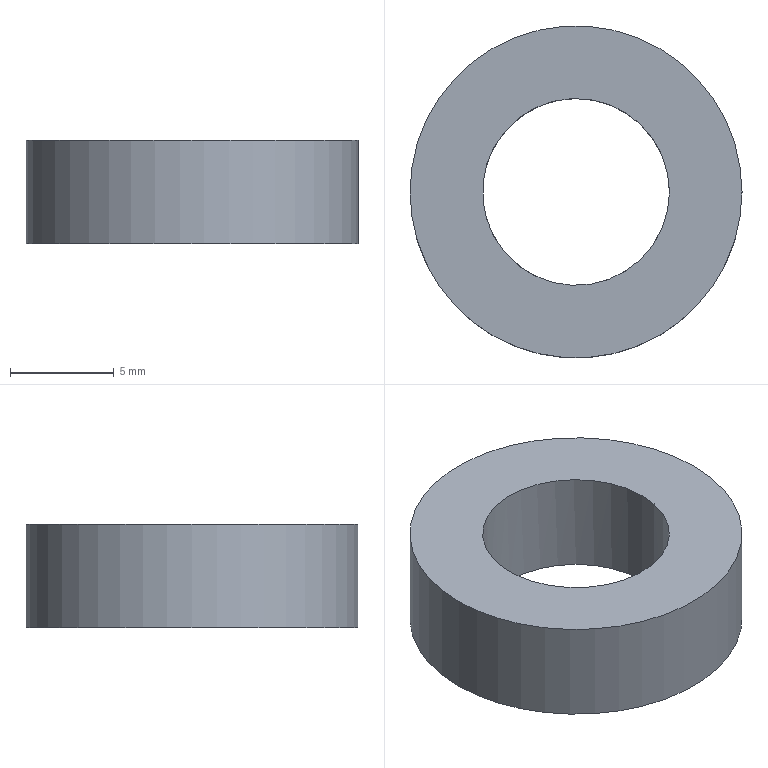Part | NX | features DIE-8 2 | 1 solid | 4 faces | box 16 x 16 x 5 mm | volume 686.728 mm3 | plane 2 | cylinder 2 | commonest cylinder face diameters 9.007 x1 16 x1
STEP:
#1=CARTESIAN_POINT('',(3222.597,-843.322,843.716));
#2=VERTEX_POINT('',#1);
#3=CARTESIAN_POINT('',(3218.094,-843.322,843.716));
#4=DIRECTION('',(0.,0.,1.));
#5=DIRECTION('',(1.,0.,0.));
#6=AXIS2_PLACEMENT_3D('',#3,#4,#5);
#7=CIRCLE('',#6,4.503);
#8=EDGE_CURVE('',#2,#2,#7,.F.);
#9=ORIENTED_EDGE('',*,*,#8,.T.);
#10=EDGE_LOOP('',(#9));
#11=FACE_BOUND('',#10,.T.);
#12=CARTESIAN_POINT('',(3226.094,-843.322,843.716));
#13=VERTEX_POINT('',#12);
#14=CARTESIAN_POINT('',(3218.094,-843.322,843.716));
#15=DIRECTION('',(0.,0.,-1.));
#16=DIRECTION('',(1.,0.,0.));
#17=AXIS2_PLACEMENT_3D('',#14,#15,#16);
#18=CIRCLE('',#17,8.);
#19=EDGE_CURVE('',#13,#13,#18,.T.);
#20=ORIENTED_EDGE('',*,*,#19,.F.);
#21=EDGE_LOOP('',(#20));
#22=FACE_BOUND('',#21,.T.);
#23=CARTESIAN_POINT('',(3218.094,-843.322,843.716));
#24=DIRECTION('',(0.,0.,1.));
#25=DIRECTION('',(1.,0.,0.));
#26=AXIS2_PLACEMENT_3D('',#23,#24,#25);
#27=PLANE('',#26);
#28=ADVANCED_FACE('',(#11,#22),#27,.T.);
#29=CARTESIAN_POINT('',(3213.59,-843.322,838.716));
#30=VERTEX_POINT('',#29);
#31=CARTESIAN_POINT('',(3218.094,-843.322,838.716));
#32=DIRECTION('',(0.,0.,-1.));
#33=DIRECTION('',(-1.,0.,0.));
#34=AXIS2_PLACEMENT_3D('',#31,#32,#33);
#35=CIRCLE('',#34,4.503);
#36=EDGE_CURVE('',#30,#30,#35,.T.);
#37=ORIENTED_EDGE('',*,*,#36,.F.);
#38=EDGE_LOOP('',(#37));
#39=FACE_BOUND('',#38,.T.);
#40=CARTESIAN_POINT('',(3226.094,-843.322,838.716));
#41=VERTEX_POINT('',#40);
#42=CARTESIAN_POINT('',(3218.094,-843.322,838.716));
#43=DIRECTION('',(0.,0.,1.));
#44=DIRECTION('',(1.,0.,0.));
#45=AXIS2_PLACEMENT_3D('',#42,#43,#44);
#46=CIRCLE('',#45,8.);
#47=EDGE_CURVE('',#41,#41,#46,.T.);
#48=ORIENTED_EDGE('',*,*,#47,.F.);
#49=EDGE_LOOP('',(#48));
#50=FACE_BOUND('',#49,.T.);
#51=CARTESIAN_POINT('',(3218.094,-843.322,838.716));
#52=DIRECTION('',(0.,0.,-1.));
#53=DIRECTION('',(-1.,0.,0.));
#54=AXIS2_PLACEMENT_3D('',#51,#52,#53);
#55=PLANE('',#54);
#56=ADVANCED_FACE('',(#39,#50),#55,.T.);
#57=ORIENTED_EDGE('',*,*,#19,.T.);
#58=EDGE_LOOP('',(#57));
#59=FACE_BOUND('',#58,.T.);
#60=ORIENTED_EDGE('',*,*,#47,.T.);
#61=EDGE_LOOP('',(#60));
#62=FACE_BOUND('',#61,.T.);
#63=CARTESIAN_POINT('',(3218.094,-843.322,838.716));
#64=DIRECTION('',(0.,0.,1.));
#65=DIRECTION('',(1.,0.,0.));
#66=AXIS2_PLACEMENT_3D('',#63,#64,#65);
#67=CYLINDRICAL_SURFACE('',#66,8.);
#68=ADVANCED_FACE('',(#59,#62),#67,.T.);
#69=ORIENTED_EDGE('',*,*,#36,.T.);
#70=EDGE_LOOP('',(#69));
#71=FACE_BOUND('',#70,.T.);
#72=ORIENTED_EDGE('',*,*,#8,.F.);
#73=EDGE_LOOP('',(#72));
#74=FACE_BOUND('',#73,.T.);
#75=CARTESIAN_POINT('',(3218.094,-843.322,843.716));
#76=DIRECTION('',(0.,0.,-1.));
#77=DIRECTION('',(1.,0.,0.));
#78=AXIS2_PLACEMENT_3D('',#75,#76,#77);
#79=CYLINDRICAL_SURFACE('',#78,4.503);
#80=ADVANCED_FACE('',(#71,#74),#79,.F.);
#81=CLOSED_SHELL('',(#28,#56,#68,#80));
#82=MANIFOLD_SOLID_BREP('',#81);
#83=(LENGTH_UNIT()NAMED_UNIT(*)SI_UNIT(.MILLI.,.METRE.));
#84=UNCERTAINTY_MEASURE_WITH_UNIT(LENGTH_MEASURE(0.00001),#83,'','');
#85=(NAMED_UNIT(*)PLANE_ANGLE_UNIT()SI_UNIT($,.RADIAN.));
#86=(NAMED_UNIT(*)SI_UNIT($,.STERADIAN.)SOLID_ANGLE_UNIT());
#87=(GEOMETRIC_REPRESENTATION_CONTEXT(3)GLOBAL_UNCERTAINTY_ASSIGNED_CONTEXT((#84))GLOBAL_UNIT_ASSIGNED_CONTEXT((#83,#85,#86))REPRESENTATION_CONTEXT('',''));
#88=ADVANCED_BREP_SHAPE_REPRESENTATION('',(#82),#87);